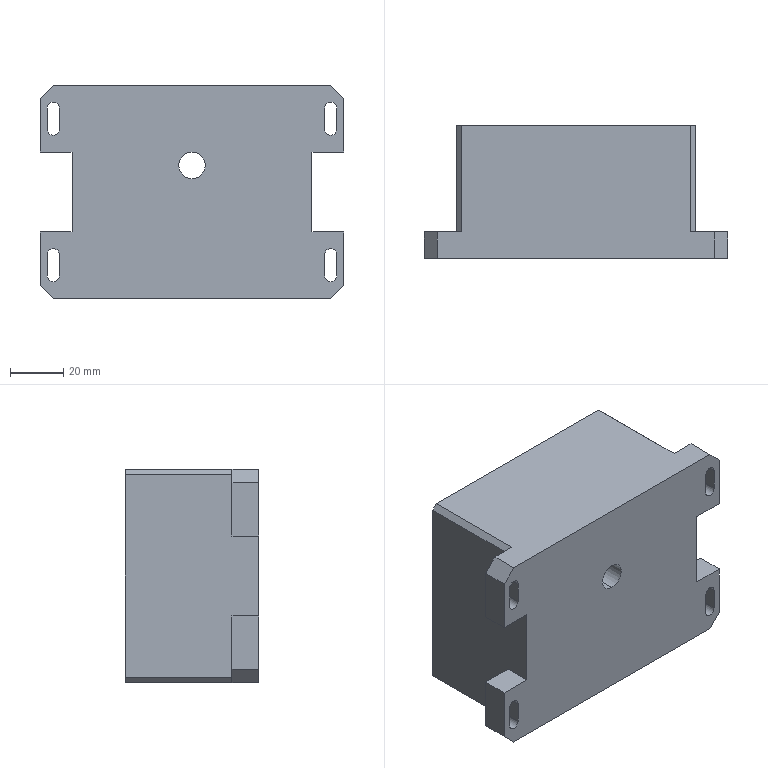Part | STEP file | PN_0014 | 1 solid | 57 faces | box 114 x 50 x 80 mm | volume 145177 mm3 | plane 39 | cylinder 18 | commonest cylinder face diameters 4.5 x12 10 x6